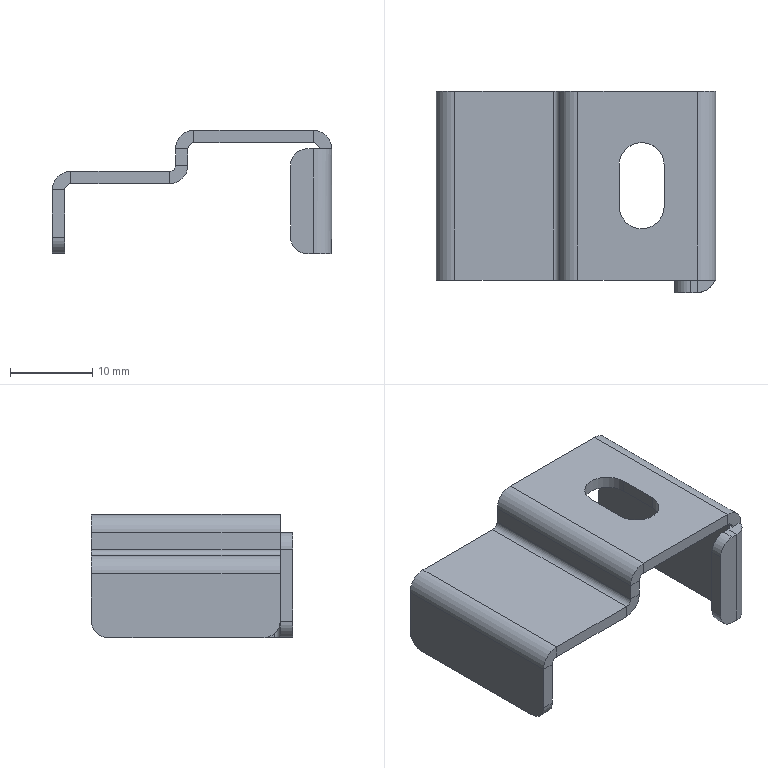Part | STEP file | 03-37 iron plate baffle A (Default) | 1 solid | 56 faces | box 34 x 24.5 x 15 mm | volume 2017 mm3 | plane 39 | cylinder 17 | commonest cylinder face diameters 1.473 x5 4 x5 4.473 x5 5.5 x2
STEP:
#1=CARTESIAN_POINT('',(9.375,-11.5,-2.237));
#2=VERTEX_POINT('',#1);
#3=CARTESIAN_POINT('',(9.5,-11.5,-2.237));
#4=VERTEX_POINT('',#3);
#5=CARTESIAN_POINT('',(8.,-11.5,-2.237));
#6=DIRECTION('',(1.,0.,0.));
#7=VECTOR('',#6,1000.);
#8=LINE('',#5,#7);
#9=EDGE_CURVE('',#2,#4,#8,.T.);
#10=ORIENTED_EDGE('',*,*,#9,.F.);
#11=CARTESIAN_POINT('',(9.5,-10.763,-2.237));
#12=VERTEX_POINT('',#11);
#13=CARTESIAN_POINT('',(7.263,-10.763,-2.237));
#14=DIRECTION('',(0.,0.,1.));
#15=DIRECTION('',(1.,0.,0.));
#16=AXIS2_PLACEMENT_3D('',#13,#14,#15);
#17=CIRCLE('',#16,2.237);
#18=EDGE_CURVE('',#2,#12,#17,.T.);
#19=ORIENTED_EDGE('',*,*,#18,.T.);
#20=CARTESIAN_POINT('',(9.5,-11.5,-2.237));
#21=DIRECTION('',(0.,1.,0.));
#22=VECTOR('',#21,1000.);
#23=LINE('',#20,#22);
#24=EDGE_CURVE('',#4,#12,#23,.T.);
#25=ORIENTED_EDGE('',*,*,#24,.F.);
#26=EDGE_LOOP('',(#10,#19,#25));
#27=FACE_OUTER_BOUND('',#26,.T.);
#28=CARTESIAN_POINT('',(8.,-11.5,-2.237));
#29=DIRECTION('',(0.,0.,-1.));
#30=DIRECTION('',(0.,1.,0.));
#31=AXIS2_PLACEMENT_3D('',#28,#29,#30);
#32=PLANE('',#31);
#33=ADVANCED_FACE('',(#27),#32,.T.);
#34=CARTESIAN_POINT('',(9.5,9.5,-15.));
#35=VERTEX_POINT('',#34);
#36=CARTESIAN_POINT('',(9.5,-10.763,-15.));
#37=VERTEX_POINT('',#36);
#38=CARTESIAN_POINT('',(9.5,-11.5,-15.));
#39=DIRECTION('',(0.,-1.,0.));
#40=VECTOR('',#39,1000.);
#41=LINE('',#38,#40);
#42=EDGE_CURVE('',#35,#37,#41,.T.);
#43=ORIENTED_EDGE('',*,*,#42,.F.);
#44=CARTESIAN_POINT('',(9.5,11.5,-13.));
#45=VERTEX_POINT('',#44);
#46=CARTESIAN_POINT('',(9.5,9.5,-13.));
#47=DIRECTION('',(1.,0.,0.));
#48=DIRECTION('',(0.,0.,-1.));
#49=AXIS2_PLACEMENT_3D('',#46,#47,#48);
#50=CIRCLE('',#49,2.);
#51=EDGE_CURVE('',#35,#45,#50,.T.);
#52=ORIENTED_EDGE('',*,*,#51,.T.);
#53=CARTESIAN_POINT('',(9.5,11.5,-2.237));
#54=VERTEX_POINT('',#53);
#55=CARTESIAN_POINT('',(9.5,11.5,-15.));
#56=DIRECTION('',(0.,0.,-1.));
#57=VECTOR('',#56,1000.);
#58=LINE('',#55,#57);
#59=EDGE_CURVE('',#54,#45,#58,.T.);
#60=ORIENTED_EDGE('',*,*,#59,.F.);
#61=CARTESIAN_POINT('',(9.5,-11.5,-2.237));
#62=DIRECTION('',(0.,-1.,0.));
#63=VECTOR('',#62,1000.);
#64=LINE('',#61,#63);
#65=EDGE_CURVE('',#54,#12,#64,.T.);
#66=ORIENTED_EDGE('',*,*,#65,.T.);
#67=CARTESIAN_POINT('',(9.5,-10.763,-2.237));
#68=DIRECTION('',(0.,0.,-1.));
#69=VECTOR('',#68,1000.);
#70=LINE('',#67,#69);
#71=EDGE_CURVE('',#12,#37,#70,.T.);
#72=ORIENTED_EDGE('',*,*,#71,.T.);
#73=EDGE_LOOP('',(#43,#52,#60,#66,#72));
#74=FACE_OUTER_BOUND('',#73,.T.);
#75=CARTESIAN_POINT('',(9.5,-11.5,-1.5));
#76=DIRECTION('',(1.,0.,0.));
#77=DIRECTION('',(0.,0.,-1.));
#78=AXIS2_PLACEMENT_3D('',#75,#76,#77);
#79=PLANE('',#78);
#80=ADVANCED_FACE('',(#74),#79,.T.);
#81=CARTESIAN_POINT('',(8.,11.5,-2.237));
#82=VERTEX_POINT('',#81);
#83=CARTESIAN_POINT('',(8.,11.5,-13.));
#84=VERTEX_POINT('',#83);
#85=CARTESIAN_POINT('',(8.,11.5,-15.));
#86=DIRECTION('',(0.,0.,-1.));
#87=VECTOR('',#86,1000.);
#88=LINE('',#85,#87);
#89=EDGE_CURVE('',#82,#84,#88,.T.);
#90=ORIENTED_EDGE('',*,*,#89,.T.);
#91=CARTESIAN_POINT('',(8.,9.5,-15.));
#92=VERTEX_POINT('',#91);
#93=CARTESIAN_POINT('',(8.,9.5,-13.));
#94=DIRECTION('',(-1.,0.,0.));
#95=DIRECTION('',(0.,0.,-1.));
#96=AXIS2_PLACEMENT_3D('',#93,#94,#95);
#97=CIRCLE('',#96,2.);
#98=EDGE_CURVE('',#84,#92,#97,.T.);
#99=ORIENTED_EDGE('',*,*,#98,.T.);
#100=CARTESIAN_POINT('',(8.,-10.763,-15.));
#101=VERTEX_POINT('',#100);
#102=CARTESIAN_POINT('',(8.,-11.5,-15.));
#103=DIRECTION('',(0.,-1.,0.));
#104=VECTOR('',#103,1000.);
#105=LINE('',#102,#104);
#106=EDGE_CURVE('',#92,#101,#105,.T.);
#107=ORIENTED_EDGE('',*,*,#106,.T.);
#108=CARTESIAN_POINT('',(8.,-10.763,-2.237));
#109=VERTEX_POINT('',#108);
#110=CARTESIAN_POINT('',(8.,-10.763,-2.237));
#111=DIRECTION('',(0.,0.,-1.));
#112=VECTOR('',#111,1000.);
#113=LINE('',#110,#112);
#114=EDGE_CURVE('',#109,#101,#113,.T.);
#115=ORIENTED_EDGE('',*,*,#114,.F.);
#116=CARTESIAN_POINT('',(8.,11.5,-2.237));
#117=DIRECTION('',(0.,-1.,0.));
#118=VECTOR('',#117,1000.);
#119=LINE('',#116,#118);
#120=EDGE_CURVE('',#82,#109,#119,.T.);
#121=ORIENTED_EDGE('',*,*,#120,.F.);
#122=EDGE_LOOP('',(#90,#99,#107,#115,#121));
#123=FACE_OUTER_BOUND('',#122,.T.);
#124=CARTESIAN_POINT('',(8.,-11.5,-1.5));
#125=DIRECTION('',(1.,0.,0.));
#126=DIRECTION('',(0.,0.,-1.));
#127=AXIS2_PLACEMENT_3D('',#124,#125,#126);
#128=PLANE('',#127);
#129=ADVANCED_FACE('',(#123),#128,.F.);
#130=CARTESIAN_POINT('',(-10.237,11.5,-6.5));
#131=VERTEX_POINT('',#130);
#132=CARTESIAN_POINT('',(-22.263,11.5,-6.5));
#133=VERTEX_POINT('',#132);
#134=CARTESIAN_POINT('',(-23.,11.5,-6.5));
#135=DIRECTION('',(-1.,0.,0.));
#136=VECTOR('',#135,1000.);
#137=LINE('',#134,#136);
#138=EDGE_CURVE('',#131,#133,#137,.T.);
#139=ORIENTED_EDGE('',*,*,#138,.T.);
#140=CARTESIAN_POINT('',(-22.263,11.5,-5.));
#141=VERTEX_POINT('',#140);
#142=CARTESIAN_POINT('',(-22.263,11.5,-6.5));
#143=DIRECTION('',(0.,0.,1.));
#144=VECTOR('',#143,1000.);
#145=LINE('',#142,#144);
#146=EDGE_CURVE('',#133,#141,#145,.T.);
#147=ORIENTED_EDGE('',*,*,#146,.T.);
#148=CARTESIAN_POINT('',(-10.237,11.5,-5.));
#149=VERTEX_POINT('',#148);
#150=CARTESIAN_POINT('',(-23.,11.5,-5.));
#151=DIRECTION('',(-1.,0.,0.));
#152=VECTOR('',#151,1000.);
#153=LINE('',#150,#152);
#154=EDGE_CURVE('',#149,#141,#153,.T.);
#155=ORIENTED_EDGE('',*,*,#154,.F.);
#156=CARTESIAN_POINT('',(-10.237,11.5,-5.));
#157=DIRECTION('',(0.,0.,-1.));
#158=VECTOR('',#157,1000.);
#159=LINE('',#156,#158);
#160=EDGE_CURVE('',#149,#131,#159,.T.);
#161=ORIENTED_EDGE('',*,*,#160,.T.);
#162=EDGE_LOOP('',(#139,#147,#155,#161));
#163=FACE_OUTER_BOUND('',#162,.T.);
#164=CARTESIAN_POINT('',(-23.,11.5,-6.5));
#165=DIRECTION('',(0.,1.,0.));
#166=DIRECTION('',(-1.,0.,0.));
#167=AXIS2_PLACEMENT_3D('',#164,#165,#166);
#168=PLANE('',#167);
#169=ADVANCED_FACE('',(#163),#168,.T.);
#170=CARTESIAN_POINT('',(-22.263,-11.5,-6.5));
#171=VERTEX_POINT('',#170);
#172=CARTESIAN_POINT('',(-10.237,-11.5,-6.5));
#173=VERTEX_POINT('',#172);
#174=CARTESIAN_POINT('',(-9.5,-11.5,-6.5));
#175=DIRECTION('',(1.,0.,0.));
#176=VECTOR('',#175,1000.);
#177=LINE('',#174,#176);
#178=EDGE_CURVE('',#171,#173,#177,.T.);
#179=ORIENTED_EDGE('',*,*,#178,.F.);
#180=CARTESIAN_POINT('',(-22.263,11.5,-6.5));
#181=DIRECTION('',(0.,-1.,0.));
#182=VECTOR('',#181,1000.);
#183=LINE('',#180,#182);
#184=EDGE_CURVE('',#133,#171,#183,.T.);
#185=ORIENTED_EDGE('',*,*,#184,.F.);
#186=ORIENTED_EDGE('',*,*,#138,.F.);
#187=CARTESIAN_POINT('',(-10.237,-11.5,-6.5));
#188=DIRECTION('',(0.,-1.,0.));
#189=VECTOR('',#188,1000.);
#190=LINE('',#187,#189);
#191=EDGE_CURVE('',#131,#173,#190,.T.);
#192=ORIENTED_EDGE('',*,*,#191,.T.);
#193=EDGE_LOOP('',(#179,#185,#186,#192));
#194=FACE_OUTER_BOUND('',#193,.T.);
#195=CARTESIAN_POINT('',(-9.5,-11.5,-6.5));
#196=DIRECTION('',(0.,0.,-1.));
#197=DIRECTION('',(-1.,0.,0.));
#198=AXIS2_PLACEMENT_3D('',#195,#196,#197);
#199=PLANE('',#198);
#200=ADVANCED_FACE('',(#194),#199,.T.);
#201=CARTESIAN_POINT('',(-22.263,-11.5,-5.));
#202=VERTEX_POINT('',#201);
#203=CARTESIAN_POINT('',(-22.263,11.5,-5.));
#204=DIRECTION('',(0.,-1.,0.));
#205=VECTOR('',#204,1000.);
#206=LINE('',#203,#205);
#207=EDGE_CURVE('',#141,#202,#206,.T.);
#208=ORIENTED_EDGE('',*,*,#207,.T.);
#209=CARTESIAN_POINT('',(-10.237,-11.5,-5.));
#210=VERTEX_POINT('',#209);
#211=CARTESIAN_POINT('',(-9.5,-11.5,-5.));
#212=DIRECTION('',(1.,0.,0.));
#213=VECTOR('',#212,1000.);
#214=LINE('',#211,#213);
#215=EDGE_CURVE('',#202,#210,#214,.T.);
#216=ORIENTED_EDGE('',*,*,#215,.T.);
#217=CARTESIAN_POINT('',(-10.237,11.5,-5.));
#218=DIRECTION('',(0.,-1.,0.));
#219=VECTOR('',#218,1000.);
#220=LINE('',#217,#219);
#221=EDGE_CURVE('',#149,#210,#220,.T.);
#222=ORIENTED_EDGE('',*,*,#221,.F.);
#223=ORIENTED_EDGE('',*,*,#154,.T.);
#224=EDGE_LOOP('',(#208,#216,#222,#223));
#225=FACE_OUTER_BOUND('',#224,.T.);
#226=CARTESIAN_POINT('',(-9.5,-11.5,-5.));
#227=DIRECTION('',(0.,0.,-1.));
#228=DIRECTION('',(-1.,0.,0.));
#229=AXIS2_PLACEMENT_3D('',#226,#227,#228);
#230=PLANE('',#229);
#231=ADVANCED_FACE('',(#225),#230,.F.);
#232=CARTESIAN_POINT('',(-9.5,-11.5,-2.237));
#233=VERTEX_POINT('',#232);
#234=CARTESIAN_POINT('',(-9.5,-11.5,-4.263));
#235=VERTEX_POINT('',#234);
#236=CARTESIAN_POINT('',(-9.5,-11.5,-5.));
#237=DIRECTION('',(0.,0.,-1.));
#238=VECTOR('',#237,1000.);
#239=LINE('',#236,#238);
#240=EDGE_CURVE('',#233,#235,#239,.T.);
#241=ORIENTED_EDGE('',*,*,#240,.T.);
#242=CARTESIAN_POINT('',(-8.,-11.5,-4.263));
#243=VERTEX_POINT('',#242);
#244=CARTESIAN_POINT('',(-9.5,-11.5,-4.263));
#245=DIRECTION('',(1.,0.,0.));
#246=VECTOR('',#245,1000.);
#247=LINE('',#244,#246);
#248=EDGE_CURVE('',#235,#243,#247,.T.);
#249=ORIENTED_EDGE('',*,*,#248,.T.);
#250=CARTESIAN_POINT('',(-8.,-11.5,-2.237));
#251=VERTEX_POINT('',#250);
#252=CARTESIAN_POINT('',(-8.,-11.5,-5.));
#253=DIRECTION('',(0.,0.,-1.));
#254=VECTOR('',#253,1000.);
#255=LINE('',#252,#254);
#256=EDGE_CURVE('',#251,#243,#255,.T.);
#257=ORIENTED_EDGE('',*,*,#256,.F.);
#258=CARTESIAN_POINT('',(-8.,-11.5,-2.237));
#259=DIRECTION('',(-1.,0.,0.));
#260=VECTOR('',#259,1000.);
#261=LINE('',#258,#260);
#262=EDGE_CURVE('',#251,#233,#261,.T.);
#263=ORIENTED_EDGE('',*,*,#262,.T.);
#264=EDGE_LOOP('',(#241,#249,#257,#263));
#265=FACE_OUTER_BOUND('',#264,.T.);
#266=CARTESIAN_POINT('',(-9.5,-11.5,-5.));
#267=DIRECTION('',(0.,-1.,0.));
#268=DIRECTION('',(1.,0.,0.));
#269=AXIS2_PLACEMENT_3D('',#266,#267,#268);
#270=PLANE('',#269);
#271=ADVANCED_FACE('',(#265),#270,.T.);
#272=CARTESIAN_POINT('',(-9.5,11.5,-4.263));
#273=VERTEX_POINT('',#272);
#274=CARTESIAN_POINT('',(-9.5,11.5,-2.237));
#275=VERTEX_POINT('',#274);
#276=CARTESIAN_POINT('',(-9.5,11.5,-1.5));
#277=DIRECTION('',(0.,0.,1.));
#278=VECTOR('',#277,1000.);
#279=LINE('',#276,#278);
#280=EDGE_CURVE('',#273,#275,#279,.T.);
#281=ORIENTED_EDGE('',*,*,#280,.F.);
#282=CARTESIAN_POINT('',(-9.5,-11.5,-4.263));
#283=DIRECTION('',(0.,1.,0.));
#284=VECTOR('',#283,1000.);
#285=LINE('',#282,#284);
#286=EDGE_CURVE('',#235,#273,#285,.T.);
#287=ORIENTED_EDGE('',*,*,#286,.F.);
#288=ORIENTED_EDGE('',*,*,#240,.F.);
#289=CARTESIAN_POINT('',(-9.5,11.5,-2.237));
#290=DIRECTION('',(0.,1.,0.));
#291=VECTOR('',#290,1000.);
#292=LINE('',#289,#291);
#293=EDGE_CURVE('',#233,#275,#292,.T.);
#294=ORIENTED_EDGE('',*,*,#293,.T.);
#295=EDGE_LOOP('',(#281,#287,#288,#294));
#296=FACE_OUTER_BOUND('',#295,.T.);
#297=CARTESIAN_POINT('',(-9.5,11.5,-1.5));
#298=DIRECTION('',(-1.,0.,0.));
#299=DIRECTION('',(0.,0.,1.));
#300=AXIS2_PLACEMENT_3D('',#297,#298,#299);
#301=PLANE('',#300);
#302=ADVANCED_FACE('',(#296),#301,.T.);
#303=CARTESIAN_POINT('',(-8.,11.5,-4.263));
#304=VERTEX_POINT('',#303);
#305=CARTESIAN_POINT('',(-8.,-11.5,-4.263));
#306=DIRECTION('',(0.,1.,0.));
#307=VECTOR('',#306,1000.);
#308=LINE('',#305,#307);
#309=EDGE_CURVE('',#243,#304,#308,.T.);
#310=ORIENTED_EDGE('',*,*,#309,.T.);
#311=CARTESIAN_POINT('',(-8.,11.5,-2.237));
#312=VERTEX_POINT('',#311);
#313=CARTESIAN_POINT('',(-8.,11.5,-1.5));
#314=DIRECTION('',(0.,0.,1.));
#315=VECTOR('',#314,1000.);
#316=LINE('',#313,#315);
#317=EDGE_CURVE('',#304,#312,#316,.T.);
#318=ORIENTED_EDGE('',*,*,#317,.T.);
#319=CARTESIAN_POINT('',(-8.,-11.5,-2.237));
#320=DIRECTION('',(0.,1.,0.));
#321=VECTOR('',#320,1000.);
#322=LINE('',#319,#321);
#323=EDGE_CURVE('',#251,#312,#322,.T.);
#324=ORIENTED_EDGE('',*,*,#323,.F.);
#325=ORIENTED_EDGE('',*,*,#256,.T.);
#326=EDGE_LOOP('',(#310,#318,#324,#325));
#327=FACE_OUTER_BOUND('',#326,.T.);
#328=CARTESIAN_POINT('',(-8.,11.5,-1.5));
#329=DIRECTION('',(-1.,0.,0.));
#330=DIRECTION('',(0.,0.,1.));
#331=AXIS2_PLACEMENT_3D('',#328,#329,#330);
#332=PLANE('',#331);
#333=ADVANCED_FACE('',(#327),#332,.F.);
#334=CARTESIAN_POINT('',(3.25,-2.5,-1.5));
#335=VERTEX_POINT('',#334);
#336=CARTESIAN_POINT('',(3.25,2.5,-1.5));
#337=VERTEX_POINT('',#336);
#338=CARTESIAN_POINT('',(3.25,-11.5,-1.5));
#339=DIRECTION('',(0.,1.,0.));
#340=VECTOR('',#339,1000.);
#341=LINE('',#338,#340);
#342=EDGE_CURVE('',#335,#337,#341,.T.);
#343=ORIENTED_EDGE('',*,*,#342,.T.);
#344=CARTESIAN_POINT('',(-2.25,2.5,-1.5));
#345=VERTEX_POINT('',#344);
#346=CARTESIAN_POINT('',(0.5,2.5,-1.5));
#347=DIRECTION('',(0.,0.,1.));
#348=DIRECTION('',(1.,0.,0.));
#349=AXIS2_PLACEMENT_3D('',#346,#347,#348);
#350=CIRCLE('',#349,2.75);
#351=EDGE_CURVE('',#337,#345,#350,.T.);
#352=ORIENTED_EDGE('',*,*,#351,.T.);
#353=CARTESIAN_POINT('',(-2.25,-2.5,-1.5));
#354=VERTEX_POINT('',#353);
#355=CARTESIAN_POINT('',(-2.25,-11.5,-1.5));
#356=DIRECTION('',(0.,-1.,0.));
#357=VECTOR('',#356,1000.);
#358=LINE('',#355,#357);
#359=EDGE_CURVE('',#345,#354,#358,.T.);
#360=ORIENTED_EDGE('',*,*,#359,.T.);
#361=CARTESIAN_POINT('',(0.5,-2.5,-1.5));
#362=DIRECTION('',(0.,0.,1.));
#363=DIRECTION('',(1.,0.,0.));
#364=AXIS2_PLACEMENT_3D('',#361,#362,#363);
#365=CIRCLE('',#364,2.75);
#366=EDGE_CURVE('',#354,#335,#365,.T.);
#367=ORIENTED_EDGE('',*,*,#366,.T.);
#368=EDGE_LOOP('',(#343,#352,#360,#367));
#369=FACE_BOUND('',#368,.T.);
#370=CARTESIAN_POINT('',(-7.263,11.5,-1.5));
#371=VERTEX_POINT('',#370);
#372=CARTESIAN_POINT('',(-7.263,-11.5,-1.5));
#373=VERTEX_POINT('',#372);
#374=CARTESIAN_POINT('',(-7.263,11.5,-1.5));
#375=DIRECTION('',(0.,-1.,0.));
#376=VECTOR('',#375,1000.);
#377=LINE('',#374,#376);
#378=EDGE_CURVE('',#371,#373,#377,.T.);
#379=ORIENTED_EDGE('',*,*,#378,.F.);
#380=CARTESIAN_POINT('',(7.263,11.5,-1.5));
#381=VERTEX_POINT('',#380);
#382=CARTESIAN_POINT('',(-8.,11.5,-1.5));
#383=DIRECTION('',(-1.,0.,0.));
#384=VECTOR('',#383,1000.);
#385=LINE('',#382,#384);
#386=EDGE_CURVE('',#381,#371,#385,.T.);
#387=ORIENTED_EDGE('',*,*,#386,.F.);
#388=CARTESIAN_POINT('',(7.263,-11.5,-1.5));
#389=VERTEX_POINT('',#388);
#390=CARTESIAN_POINT('',(7.263,-11.5,-1.5));
#391=DIRECTION('',(0.,1.,0.));
#392=VECTOR('',#391,1000.);
#393=LINE('',#390,#392);
#394=EDGE_CURVE('',#389,#381,#393,.T.);
#395=ORIENTED_EDGE('',*,*,#394,.F.);
#396=CARTESIAN_POINT('',(-8.,-11.5,-1.5));
#397=DIRECTION('',(1.,0.,0.));
#398=VECTOR('',#397,1000.);
#399=LINE('',#396,#398);
#400=EDGE_CURVE('',#373,#389,#399,.T.);
#401=ORIENTED_EDGE('',*,*,#400,.F.);
#402=EDGE_LOOP('',(#379,#387,#395,#401));
#403=FACE_OUTER_BOUND('',#402,.T.);
#404=CARTESIAN_POINT('',(8.,-11.5,-1.5));
#405=DIRECTION('',(0.,0.,1.));
#406=DIRECTION('',(1.,0.,0.));
#407=AXIS2_PLACEMENT_3D('',#404,#405,#406);
#408=PLANE('',#407);
#409=ADVANCED_FACE('',(#369,#403),#408,.F.);
#410=CARTESIAN_POINT('',(3.25,2.5,0.));
#411=VERTEX_POINT('',#410);
#412=CARTESIAN_POINT('',(-2.25,2.5,0.));
#413=VERTEX_POINT('',#412);
#414=CARTESIAN_POINT('',(0.5,2.5,0.));
#415=DIRECTION('',(0.,0.,1.));
#416=DIRECTION('',(1.,0.,0.));
#417=AXIS2_PLACEMENT_3D('',#414,#415,#416);
#418=CIRCLE('',#417,2.75);
#419=EDGE_CURVE('',#411,#413,#418,.T.);
#420=ORIENTED_EDGE('',*,*,#419,.F.);
#421=CARTESIAN_POINT('',(3.25,-2.5,0.));
#422=VERTEX_POINT('',#421);
#423=CARTESIAN_POINT('',(3.25,2.5,0.));
#424=DIRECTION('',(0.,1.,0.));
#425=VECTOR('',#424,1000.);
#426=LINE('',#423,#425);
#427=EDGE_CURVE('',#422,#411,#426,.T.);
#428=ORIENTED_EDGE('',*,*,#427,.F.);
#429=CARTESIAN_POINT('',(-2.25,-2.5,0.));
#430=VERTEX_POINT('',#429);
#431=CARTESIAN_POINT('',(0.5,-2.5,0.));
#432=DIRECTION('',(0.,0.,1.));
#433=DIRECTION('',(1.,0.,0.));
#434=AXIS2_PLACEMENT_3D('',#431,#432,#433);
#435=CIRCLE('',#434,2.75);
#436=EDGE_CURVE('',#430,#422,#435,.T.);
#437=ORIENTED_EDGE('',*,*,#436,.F.);
#438=CARTESIAN_POINT('',(-2.25,2.5,0.));
#439=DIRECTION('',(0.,-1.,0.));
#440=VECTOR('',#439,1000.);
#441=LINE('',#438,#440);
#442=EDGE_CURVE('',#413,#430,#441,.T.);
#443=ORIENTED_EDGE('',*,*,#442,.F.);
#444=EDGE_LOOP('',(#420,#428,#437,#443));
#445=FACE_BOUND('',#444,.T.);
#446=CARTESIAN_POINT('',(7.263,11.5,0.));
#447=VERTEX_POINT('',#446);
#448=CARTESIAN_POINT('',(-7.263,11.5,0.));
#449=VERTEX_POINT('',#448);
#450=CARTESIAN_POINT('',(-8.,11.5,0.));
#451=DIRECTION('',(-1.,0.,0.));
#452=VECTOR('',#451,1000.);
#453=LINE('',#450,#452);
#454=EDGE_CURVE('',#447,#449,#453,.T.);
#455=ORIENTED_EDGE('',*,*,#454,.T.);
#456=CARTESIAN_POINT('',(-7.263,-11.5,0.));
#457=VERTEX_POINT('',#456);
#458=CARTESIAN_POINT('',(-7.263,11.5,0.));
#459=DIRECTION('',(0.,-1.,0.));
#460=VECTOR('',#459,1000.);
#461=LINE('',#458,#460);
#462=EDGE_CURVE('',#449,#457,#461,.T.);
#463=ORIENTED_EDGE('',*,*,#462,.T.);
#464=CARTESIAN_POINT('',(7.263,-11.5,0.));
#465=VERTEX_POINT('',#464);
#466=CARTESIAN_POINT('',(-8.,-11.5,0.));
#467=DIRECTION('',(1.,0.,0.));
#468=VECTOR('',#467,1000.);
#469=LINE('',#466,#468);
#470=EDGE_CURVE('',#457,#465,#469,.T.);
#471=ORIENTED_EDGE('',*,*,#470,.T.);
#472=CARTESIAN_POINT('',(7.263,-11.5,0.));
#473=DIRECTION('',(0.,1.,0.));
#474=VECTOR('',#473,1000.);
#475=LINE('',#472,#474);
#476=EDGE_CURVE('',#465,#447,#475,.T.);
#477=ORIENTED_EDGE('',*,*,#476,.T.);
#478=EDGE_LOOP('',(#455,#463,#471,#477));
#479=FACE_OUTER_BOUND('',#478,.T.);
#480=CARTESIAN_POINT('',(8.,-11.5,0.));
#481=DIRECTION('',(0.,0.,1.));
#482=DIRECTION('',(1.,0.,0.));
#483=AXIS2_PLACEMENT_3D('',#480,#481,#482);
#484=PLANE('',#483);
#485=ADVANCED_FACE('',(#445,#479),#484,.T.);
#486=ORIENTED_EDGE('',*,*,#386,.T.);
#487=CARTESIAN_POINT('',(-7.263,11.5,-1.5));
#488=DIRECTION('',(0.,0.,1.));
#489=VECTOR('',#488,1000.);
#490=LINE('',#487,#489);
#491=EDGE_CURVE('',#371,#449,#490,.T.);
#492=ORIENTED_EDGE('',*,*,#491,.T.);
#493=ORIENTED_EDGE('',*,*,#454,.F.);
#494=CARTESIAN_POINT('',(7.263,11.5,-1.5));
#495=DIRECTION('',(0.,0.,1.));
#496=VECTOR('',#495,1000.);
#497=LINE('',#494,#496);
#498=EDGE_CURVE('',#381,#447,#497,.T.);
#499=ORIENTED_EDGE('',*,*,#498,.F.);
#500=EDGE_LOOP('',(#486,#492,#493,#499));
#501=FACE_OUTER_BOUND('',#500,.T.);
#502=CARTESIAN_POINT('',(-8.,11.5,-1.5));
#503=DIRECTION('',(0.,1.,0.));
#504=DIRECTION('',(0.,0.,1.));
#505=AXIS2_PLACEMENT_3D('',#502,#503,#504);
#506=PLANE('',#505);
#507=ADVANCED_FACE('',(#501),#506,.T.);
#508=CARTESIAN_POINT('',(-7.263,-11.5,-1.5));
#509=DIRECTION('',(0.,0.,1.));
#510=VECTOR('',#509,1000.);
#511=LINE('',#508,#510);
#512=EDGE_CURVE('',#373,#457,#511,.T.);
#513=ORIENTED_EDGE('',*,*,#512,.F.);
#514=ORIENTED_EDGE('',*,*,#400,.T.);
#515=CARTESIAN_POINT('',(7.263,-11.5,-1.5));
#516=DIRECTION('',(0.,0.,1.));
#517=VECTOR('',#516,1000.);
#518=LINE('',#515,#517);
#519=EDGE_CURVE('',#389,#465,#518,.T.);
#520=ORIENTED_EDGE('',*,*,#519,.T.);
#521=ORIENTED_EDGE('',*,*,#470,.F.);
#522=EDGE_LOOP('',(#513,#514,#520,#521));
#523=FACE_OUTER_BOUND('',#522,.T.);
#524=CARTESIAN_POINT('',(-8.,-11.5,-1.5));
#525=DIRECTION('',(0.,-1.,0.));
#526=DIRECTION('',(0.,0.,-1.));
#527=AXIS2_PLACEMENT_3D('',#524,#525,#526);
#528=PLANE('',#527);
#529=ADVANCED_FACE('',(#523),#528,.T.);
#530=CARTESIAN_POINT('',(8.,11.5,-2.237));
#531=DIRECTION('',(1.,0.,0.));
#532=VECTOR('',#531,1000.);
#533=LINE('',#530,#532);
#534=EDGE_CURVE('',#82,#54,#533,.T.);
#535=ORIENTED_EDGE('',*,*,#534,.F.);
#536=CARTESIAN_POINT('',(7.263,11.5,-2.237));
#537=DIRECTION('',(0.,1.,0.));
#538=DIRECTION('',(0.,0.,-1.));
#539=AXIS2_PLACEMENT_3D('',#536,#537,#538);
#540=CIRCLE('',#539,0.7366);
#541=EDGE_CURVE('',#381,#82,#540,.T.);
#542=ORIENTED_EDGE('',*,*,#541,.F.);
#543=ORIENTED_EDGE('',*,*,#498,.T.);
#544=CARTESIAN_POINT('',(7.263,11.5,-2.237));
#545=DIRECTION('',(0.,1.,0.));
#546=DIRECTION('',(0.,0.,-1.));
#547=AXIS2_PLACEMENT_3D('',#544,#545,#546);
#548=CIRCLE('',#547,2.237);
#549=EDGE_CURVE('',#447,#54,#548,.T.);
#550=ORIENTED_EDGE('',*,*,#549,.T.);
#551=EDGE_LOOP('',(#535,#542,#543,#550));
#552=FACE_OUTER_BOUND('',#551,.T.);
#553=CARTESIAN_POINT('',(7.263,11.5,-2.237));
#554=DIRECTION('',(0.,1.,0.));
#555=DIRECTION('',(0.,0.,1.));
#556=AXIS2_PLACEMENT_3D('',#553,#554,#555);
#557=PLANE('',#556);
#558=ADVANCED_FACE('',(#552),#557,.T.);
#559=CARTESIAN_POINT('',(8.,-11.5,-2.237));
#560=VERTEX_POINT('',#559);
#561=CARTESIAN_POINT('',(7.263,-11.5,-2.237));
#562=DIRECTION('',(0.,-1.,0.));
#563=DIRECTION('',(0.,0.,-1.));
#564=AXIS2_PLACEMENT_3D('',#561,#562,#563);
#565=CIRCLE('',#564,0.7366);
#566=EDGE_CURVE('',#560,#389,#565,.T.);
#567=ORIENTED_EDGE('',*,*,#566,.F.);
#568=CARTESIAN_POINT('',(8.,-11.5,-2.237));
#569=DIRECTION('',(1.,0.,0.));
#570=VECTOR('',#569,1000.);
#571=LINE('',#568,#570);
#572=EDGE_CURVE('',#560,#2,#571,.T.);
#573=ORIENTED_EDGE('',*,*,#572,.T.);
#574=ORIENTED_EDGE('',*,*,#9,.T.);
#575=CARTESIAN_POINT('',(7.263,-11.5,-2.237));
#576=DIRECTION('',(0.,-1.,0.));
#577=DIRECTION('',(0.,0.,-1.));
#578=AXIS2_PLACEMENT_3D('',#575,#576,#577);
#579=CIRCLE('',#578,2.237);
#580=EDGE_CURVE('',#4,#465,#579,.T.);
#581=ORIENTED_EDGE('',*,*,#580,.T.);
#582=ORIENTED_EDGE('',*,*,#519,.F.);
#583=EDGE_LOOP('',(#567,#573,#574,#581,#582));
#584=FACE_OUTER_BOUND('',#583,.T.);
#585=CARTESIAN_POINT('',(7.263,-11.5,-2.237));
#586=DIRECTION('',(0.,1.,0.));
#587=DIRECTION('',(0.,0.,1.));
#588=AXIS2_PLACEMENT_3D('',#585,#586,#587);
#589=PLANE('',#588);
#590=ADVANCED_FACE('',(#584),#589,.F.);
#591=ORIENTED_EDGE('',*,*,#476,.F.);
#592=ORIENTED_EDGE('',*,*,#580,.F.);
#593=ORIENTED_EDGE('',*,*,#24,.T.);
#594=ORIENTED_EDGE('',*,*,#65,.F.);
#595=ORIENTED_EDGE('',*,*,#549,.F.);
#596=EDGE_LOOP('',(#591,#592,#593,#594,#595));
#597=FACE_OUTER_BOUND('',#596,.T.);
#598=CARTESIAN_POINT('',(7.263,-11.5,-2.237));
#599=DIRECTION('',(0.,-1.,0.));
#600=DIRECTION('',(1.,0.,0.));
#601=AXIS2_PLACEMENT_3D('',#598,#599,#600);
#602=CYLINDRICAL_SURFACE('',#601,2.237);
#603=ADVANCED_FACE('',(#597),#602,.T.);
#604=ORIENTED_EDGE('',*,*,#394,.T.);
#605=ORIENTED_EDGE('',*,*,#541,.T.);
#606=ORIENTED_EDGE('',*,*,#120,.T.);
#607=CARTESIAN_POINT('',(8.,-11.5,-2.237));
#608=DIRECTION('',(0.,1.,0.));
#609=VECTOR('',#608,1000.);
#610=LINE('',#607,#609);
#611=EDGE_CURVE('',#560,#109,#610,.T.);
#612=ORIENTED_EDGE('',*,*,#611,.F.);
#613=ORIENTED_EDGE('',*,*,#566,.T.);
#614=EDGE_LOOP('',(#604,#605,#606,#612,#613));
#615=FACE_OUTER_BOUND('',#614,.T.);
#616=CARTESIAN_POINT('',(7.263,-11.5,-2.237));
#617=DIRECTION('',(0.,-1.,0.));
#618=DIRECTION('',(1.,0.,0.));
#619=AXIS2_PLACEMENT_3D('',#616,#617,#618);
#620=CYLINDRICAL_SURFACE('',#619,0.7366);
#621=ADVANCED_FACE('',(#615),#620,.F.);
#622=ORIENTED_EDGE('',*,*,#59,.T.);
#623=CARTESIAN_POINT('',(9.5,11.5,-13.));
#624=DIRECTION('',(-1.,0.,0.));
#625=VECTOR('',#624,1000.);
#626=LINE('',#623,#625);
#627=EDGE_CURVE('',#45,#84,#626,.T.);
#628=ORIENTED_EDGE('',*,*,#627,.T.);
#629=ORIENTED_EDGE('',*,*,#89,.F.);
#630=ORIENTED_EDGE('',*,*,#534,.T.);
#631=EDGE_LOOP('',(#622,#628,#629,#630));
#632=FACE_OUTER_BOUND('',#631,.T.);
#633=CARTESIAN_POINT('',(9.5,11.5,-15.));
#634=DIRECTION('',(0.,1.,0.));
#635=DIRECTION('',(-1.,0.,0.));
#636=AXIS2_PLACEMENT_3D('',#633,#634,#635);
#637=PLANE('',#636);
#638=ADVANCED_FACE('',(#632),#637,.T.);
#639=ORIENTED_EDGE('',*,*,#106,.F.);
#640=CARTESIAN_POINT('',(9.5,9.5,-15.));
#641=DIRECTION('',(1.,0.,0.));
#642=VECTOR('',#641,1000.);
#643=LINE('',#640,#642);
#644=EDGE_CURVE('',#92,#35,#643,.T.);
#645=ORIENTED_EDGE('',*,*,#644,.T.);
#646=ORIENTED_EDGE('',*,*,#42,.T.);
#647=CARTESIAN_POINT('',(8.,-10.763,-15.));
#648=DIRECTION('',(1.,0.,0.));
#649=VECTOR('',#648,1000.);
#650=LINE('',#647,#649);
#651=EDGE_CURVE('',#101,#37,#650,.T.);
#652=ORIENTED_EDGE('',*,*,#651,.F.);
#653=EDGE_LOOP('',(#639,#645,#646,#652));
#654=FACE_OUTER_BOUND('',#653,.T.);
#655=CARTESIAN_POINT('',(9.5,-11.5,-15.));
#656=DIRECTION('',(0.,0.,-1.));
#657=DIRECTION('',(-1.,0.,0.));
#658=AXIS2_PLACEMENT_3D('',#655,#656,#657);
#659=PLANE('',#658);
#660=ADVANCED_FACE('',(#654),#659,.T.);
#661=ORIENTED_EDGE('',*,*,#262,.F.);
#662=CARTESIAN_POINT('',(-7.263,-11.5,-2.237));
#663=DIRECTION('',(0.,-1.,0.));
#664=DIRECTION('',(0.,0.,1.));
#665=AXIS2_PLACEMENT_3D('',#662,#663,#664);
#666=CIRCLE('',#665,0.7366);
#667=EDGE_CURVE('',#373,#251,#666,.T.);
#668=ORIENTED_EDGE('',*,*,#667,.F.);
#669=ORIENTED_EDGE('',*,*,#512,.T.);
#670=CARTESIAN_POINT('',(-7.263,-11.5,-2.237));
#671=DIRECTION('',(0.,-1.,0.));
#672=DIRECTION('',(0.,0.,1.));
#673=AXIS2_PLACEMENT_3D('',#670,#671,#672);
#674=CIRCLE('',#673,2.237);
#675=EDGE_CURVE('',#457,#233,#674,.T.);
#676=ORIENTED_EDGE('',*,*,#675,.T.);
#677=EDGE_LOOP('',(#661,#668,#669,#676));
#678=FACE_OUTER_BOUND('',#677,.T.);
#679=CARTESIAN_POINT('',(-7.263,-11.5,-2.237));
#680=DIRECTION('',(0.,-1.,0.));
#681=DIRECTION('',(0.,0.,-1.));
#682=AXIS2_PLACEMENT_3D('',#679,#680,#681);
#683=PLANE('',#682);
#684=ADVANCED_FACE('',(#678),#683,.T.);
#685=CARTESIAN_POINT('',(-7.263,11.5,-2.237));
#686=DIRECTION('',(0.,1.,0.));
#687=DIRECTION('',(0.,0.,1.));
#688=AXIS2_PLACEMENT_3D('',#685,#686,#687);
#689=CIRCLE('',#688,0.7366);
#690=EDGE_CURVE('',#312,#371,#689,.T.);
#691=ORIENTED_EDGE('',*,*,#690,.F.);
#692=CARTESIAN_POINT('',(-8.,11.5,-2.237));
#693=DIRECTION('',(-1.,0.,0.));
#694=VECTOR('',#693,1000.);
#695=LINE('',#692,#694);
#696=EDGE_CURVE('',#312,#275,#695,.T.);
#697=ORIENTED_EDGE('',*,*,#696,.T.);
#698=CARTESIAN_POINT('',(-7.263,11.5,-2.237));
#699=DIRECTION('',(0.,1.,0.));
#700=DIRECTION('',(0.,0.,1.));
#701=AXIS2_PLACEMENT_3D('',#698,#699,#700);
#702=CIRCLE('',#701,2.237);
#703=EDGE_CURVE('',#275,#449,#702,.T.);
#704=ORIENTED_EDGE('',*,*,#703,.T.);
#705=ORIENTED_EDGE('',*,*,#491,.F.);
#706=EDGE_LOOP('',(#691,#697,#704,#705));
#707=FACE_OUTER_BOUND('',#706,.T.);
#708=CARTESIAN_POINT('',(-7.263,11.5,-2.237));
#709=DIRECTION('',(0.,-1.,0.));
#710=DIRECTION('',(0.,0.,-1.));
#711=AXIS2_PLACEMENT_3D('',#708,#709,#710);
#712=PLANE('',#711);
#713=ADVANCED_FACE('',(#707),#712,.F.);
#714=ORIENTED_EDGE('',*,*,#462,.F.);
#715=ORIENTED_EDGE('',*,*,#703,.F.);
#716=ORIENTED_EDGE('',*,*,#293,.F.);
#717=ORIENTED_EDGE('',*,*,#675,.F.);
#718=EDGE_LOOP('',(#714,#715,#716,#717));
#719=FACE_OUTER_BOUND('',#718,.T.);
#720=CARTESIAN_POINT('',(-7.263,11.5,-2.237));
#721=DIRECTION('',(0.,1.,0.));
#722=DIRECTION('',(-1.,0.,0.));
#723=AXIS2_PLACEMENT_3D('',#720,#721,#722);
#724=CYLINDRICAL_SURFACE('',#723,2.237);
#725=ADVANCED_FACE('',(#719),#724,.T.);
#726=ORIENTED_EDGE('',*,*,#378,.T.);
#727=ORIENTED_EDGE('',*,*,#667,.T.);
#728=ORIENTED_EDGE('',*,*,#323,.T.);
#729=ORIENTED_EDGE('',*,*,#690,.T.);
#730=EDGE_LOOP('',(#726,#727,#728,#729));
#731=FACE_OUTER_BOUND('',#730,.T.);
#732=CARTESIAN_POINT('',(-7.263,11.5,-2.237));
#733=DIRECTION('',(0.,1.,0.));
#734=DIRECTION('',(-1.,0.,0.));
#735=AXIS2_PLACEMENT_3D('',#732,#733,#734);
#736=CYLINDRICAL_SURFACE('',#735,0.7366);
#737=ADVANCED_FACE('',(#731),#736,.F.);
#738=CARTESIAN_POINT('',(-9.5,11.5,-4.263));
#739=DIRECTION('',(1.,0.,0.));
#740=VECTOR('',#739,1000.);
#741=LINE('',#738,#740);
#742=EDGE_CURVE('',#273,#304,#741,.T.);
#743=ORIENTED_EDGE('',*,*,#742,.F.);
#744=ORIENTED_EDGE('',*,*,#280,.T.);
#745=ORIENTED_EDGE('',*,*,#696,.F.);
#746=ORIENTED_EDGE('',*,*,#317,.F.);
#747=EDGE_LOOP('',(#743,#744,#745,#746));
#748=FACE_OUTER_BOUND('',#747,.T.);
#749=CARTESIAN_POINT('',(-9.5,11.5,-1.5));
#750=DIRECTION('',(0.,1.,0.));
#751=DIRECTION('',(-1.,0.,0.));
#752=AXIS2_PLACEMENT_3D('',#749,#750,#751);
#753=PLANE('',#752);
#754=ADVANCED_FACE('',(#748),#753,.T.);
#755=ORIENTED_EDGE('',*,*,#160,.F.);
#756=CARTESIAN_POINT('',(-10.237,11.5,-4.263));
#757=DIRECTION('',(0.,1.,0.));
#758=DIRECTION('',(0.,0.,-1.));
#759=AXIS2_PLACEMENT_3D('',#756,#757,#758);
#760=CIRCLE('',#759,0.7366);
#761=EDGE_CURVE('',#273,#149,#760,.T.);
#762=ORIENTED_EDGE('',*,*,#761,.F.);
#763=ORIENTED_EDGE('',*,*,#742,.T.);
#764=CARTESIAN_POINT('',(-10.237,11.5,-4.263));
#765=DIRECTION('',(0.,1.,0.));
#766=DIRECTION('',(0.,0.,-1.));
#767=AXIS2_PLACEMENT_3D('',#764,#765,#766);
#768=CIRCLE('',#767,2.237);
#769=EDGE_CURVE('',#304,#131,#768,.T.);
#770=ORIENTED_EDGE('',*,*,#769,.T.);
#771=EDGE_LOOP('',(#755,#762,#763,#770));
#772=FACE_OUTER_BOUND('',#771,.T.);
#773=CARTESIAN_POINT('',(-10.237,11.5,-4.263));
#774=DIRECTION('',(0.,1.,0.));
#775=DIRECTION('',(0.,0.,1.));
#776=AXIS2_PLACEMENT_3D('',#773,#774,#775);
#777=PLANE('',#776);
#778=ADVANCED_FACE('',(#772),#777,.T.);
#779=CARTESIAN_POINT('',(-10.237,-11.5,-4.263));
#780=DIRECTION('',(0.,-1.,0.));
#781=DIRECTION('',(0.,0.,-1.));
#782=AXIS2_PLACEMENT_3D('',#779,#780,#781);
#783=CIRCLE('',#782,0.7366);
#784=EDGE_CURVE('',#210,#235,#783,.T.);
#785=ORIENTED_EDGE('',*,*,#784,.F.);
#786=CARTESIAN_POINT('',(-10.237,-11.5,-5.));
#787=DIRECTION('',(0.,0.,-1.));
#788=VECTOR('',#787,1000.);
#789=LINE('',#786,#788);
#790=EDGE_CURVE('',#210,#173,#789,.T.);
#791=ORIENTED_EDGE('',*,*,#790,.T.);
#792=CARTESIAN_POINT('',(-10.237,-11.5,-4.263));
#793=DIRECTION('',(0.,-1.,0.));
#794=DIRECTION('',(0.,0.,-1.));
#795=AXIS2_PLACEMENT_3D('',#792,#793,#794);
#796=CIRCLE('',#795,2.237);
#797=EDGE_CURVE('',#173,#243,#796,.T.);
#798=ORIENTED_EDGE('',*,*,#797,.T.);
#799=ORIENTED_EDGE('',*,*,#248,.F.);
#800=EDGE_LOOP('',(#785,#791,#798,#799));
#801=FACE_OUTER_BOUND('',#800,.T.);
#802=CARTESIAN_POINT('',(-10.237,-11.5,-4.263));
#803=DIRECTION('',(0.,1.,0.));
#804=DIRECTION('',(0.,0.,1.));
#805=AXIS2_PLACEMENT_3D('',#802,#803,#804);
#806=PLANE('',#805);
#807=ADVANCED_FACE('',(#801),#806,.F.);
#808=ORIENTED_EDGE('',*,*,#309,.F.);
#809=ORIENTED_EDGE('',*,*,#797,.F.);
#810=ORIENTED_EDGE('',*,*,#191,.F.);
#811=ORIENTED_EDGE('',*,*,#769,.F.);
#812=EDGE_LOOP('',(#808,#809,#810,#811));
#813=FACE_OUTER_BOUND('',#812,.T.);
#814=CARTESIAN_POINT('',(-10.237,-11.5,-4.263));
#815=DIRECTION('',(0.,-1.,0.));
#816=DIRECTION('',(0.,0.,-1.));
#817=AXIS2_PLACEMENT_3D('',#814,#815,#816);
#818=CYLINDRICAL_SURFACE('',#817,2.237);
#819=ADVANCED_FACE('',(#813),#818,.T.);
#820=ORIENTED_EDGE('',*,*,#286,.T.);
#821=ORIENTED_EDGE('',*,*,#761,.T.);
#822=ORIENTED_EDGE('',*,*,#221,.T.);
#823=ORIENTED_EDGE('',*,*,#784,.T.);
#824=EDGE_LOOP('',(#820,#821,#822,#823));
#825=FACE_OUTER_BOUND('',#824,.T.);
#826=CARTESIAN_POINT('',(-10.237,-11.5,-4.263));
#827=DIRECTION('',(0.,-1.,0.));
#828=DIRECTION('',(0.,0.,-1.));
#829=AXIS2_PLACEMENT_3D('',#826,#827,#828);
#830=CYLINDRICAL_SURFACE('',#829,0.7366);
#831=ADVANCED_FACE('',(#825),#830,.F.);
#832=CARTESIAN_POINT('',(-22.263,-11.5,-6.5));
#833=DIRECTION('',(0.,0.,1.));
#834=VECTOR('',#833,1000.);
#835=LINE('',#832,#834);
#836=EDGE_CURVE('',#171,#202,#835,.T.);
#837=ORIENTED_EDGE('',*,*,#836,.F.);
#838=ORIENTED_EDGE('',*,*,#178,.T.);
#839=ORIENTED_EDGE('',*,*,#790,.F.);
#840=ORIENTED_EDGE('',*,*,#215,.F.);
#841=EDGE_LOOP('',(#837,#838,#839,#840));
#842=FACE_OUTER_BOUND('',#841,.T.);
#843=CARTESIAN_POINT('',(-9.5,-11.5,-6.5));
#844=DIRECTION('',(0.,-1.,0.));
#845=DIRECTION('',(1.,0.,0.));
#846=AXIS2_PLACEMENT_3D('',#843,#844,#845);
#847=PLANE('',#846);
#848=ADVANCED_FACE('',(#842),#847,.T.);
#849=CARTESIAN_POINT('',(-23.,-11.5,-7.237));
#850=VERTEX_POINT('',#849);
#851=CARTESIAN_POINT('',(-24.5,-11.5,-7.237));
#852=VERTEX_POINT('',#851);
#853=CARTESIAN_POINT('',(-23.,-11.5,-7.237));
#854=DIRECTION('',(-1.,0.,0.));
#855=VECTOR('',#854,1000.);
#856=LINE('',#853,#855);
#857=EDGE_CURVE('',#850,#852,#856,.T.);
#858=ORIENTED_EDGE('',*,*,#857,.F.);
#859=CARTESIAN_POINT('',(-22.263,-11.5,-7.237));
#860=DIRECTION('',(0.,-1.,0.));
#861=DIRECTION('',(0.,0.,1.));
#862=AXIS2_PLACEMENT_3D('',#859,#860,#861);
#863=CIRCLE('',#862,0.7366);
#864=EDGE_CURVE('',#171,#850,#863,.T.);
#865=ORIENTED_EDGE('',*,*,#864,.F.);
#866=ORIENTED_EDGE('',*,*,#836,.T.);
#867=CARTESIAN_POINT('',(-22.263,-11.5,-7.237));
#868=DIRECTION('',(0.,-1.,0.));
#869=DIRECTION('',(0.,0.,1.));
#870=AXIS2_PLACEMENT_3D('',#867,#868,#869);
#871=CIRCLE('',#870,2.237);
#872=EDGE_CURVE('',#202,#852,#871,.T.);
#873=ORIENTED_EDGE('',*,*,#872,.T.);
#874=EDGE_LOOP('',(#858,#865,#866,#873));
#875=FACE_OUTER_BOUND('',#874,.T.);
#876=CARTESIAN_POINT('',(-22.263,-11.5,-7.237));
#877=DIRECTION('',(0.,-1.,0.));
#878=DIRECTION('',(0.,0.,-1.));
#879=AXIS2_PLACEMENT_3D('',#876,#877,#878);
#880=PLANE('',#879);
#881=ADVANCED_FACE('',(#875),#880,.T.);
#882=CARTESIAN_POINT('',(-23.,11.5,-7.237));
#883=VERTEX_POINT('',#882);
#884=CARTESIAN_POINT('',(-22.263,11.5,-7.237));
#885=DIRECTION('',(0.,1.,0.));
#886=DIRECTION('',(0.,0.,1.));
#887=AXIS2_PLACEMENT_3D('',#884,#885,#886);
#888=CIRCLE('',#887,0.7366);
#889=EDGE_CURVE('',#883,#133,#888,.T.);
#890=ORIENTED_EDGE('',*,*,#889,.F.);
#891=CARTESIAN_POINT('',(-24.5,11.5,-7.237));
#892=VERTEX_POINT('',#891);
#893=CARTESIAN_POINT('',(-23.,11.5,-7.237));
#894=DIRECTION('',(-1.,0.,0.));
#895=VECTOR('',#894,1000.);
#896=LINE('',#893,#895);
#897=EDGE_CURVE('',#883,#892,#896,.T.);
#898=ORIENTED_EDGE('',*,*,#897,.T.);
#899=CARTESIAN_POINT('',(-22.263,11.5,-7.237));
#900=DIRECTION('',(0.,1.,0.));
#901=DIRECTION('',(0.,0.,1.));
#902=AXIS2_PLACEMENT_3D('',#899,#900,#901);
#903=CIRCLE('',#902,2.237);
#904=EDGE_CURVE('',#892,#141,#903,.T.);
#905=ORIENTED_EDGE('',*,*,#904,.T.);
#906=ORIENTED_EDGE('',*,*,#146,.F.);
#907=EDGE_LOOP('',(#890,#898,#905,#906));
#908=FACE_OUTER_BOUND('',#907,.T.);
#909=CARTESIAN_POINT('',(-22.263,11.5,-7.237));
#910=DIRECTION('',(0.,-1.,0.));
#911=DIRECTION('',(0.,0.,-1.));
#912=AXIS2_PLACEMENT_3D('',#909,#910,#911);
#913=PLANE('',#912);
#914=ADVANCED_FACE('',(#908),#913,.F.);
#915=ORIENTED_EDGE('',*,*,#207,.F.);
#916=ORIENTED_EDGE('',*,*,#904,.F.);
#917=CARTESIAN_POINT('',(-24.5,11.5,-7.237));
#918=DIRECTION('',(0.,1.,0.));
#919=VECTOR('',#918,1000.);
#920=LINE('',#917,#919);
#921=EDGE_CURVE('',#852,#892,#920,.T.);
#922=ORIENTED_EDGE('',*,*,#921,.F.);
#923=ORIENTED_EDGE('',*,*,#872,.F.);
#924=EDGE_LOOP('',(#915,#916,#922,#923));
#925=FACE_OUTER_BOUND('',#924,.T.);
#926=CARTESIAN_POINT('',(-22.263,11.5,-7.237));
#927=DIRECTION('',(0.,1.,0.));
#928=DIRECTION('',(-1.,0.,0.));
#929=AXIS2_PLACEMENT_3D('',#926,#927,#928);
#930=CYLINDRICAL_SURFACE('',#929,2.237);
#931=ADVANCED_FACE('',(#925),#930,.T.);
#932=ORIENTED_EDGE('',*,*,#184,.T.);
#933=ORIENTED_EDGE('',*,*,#864,.T.);
#934=CARTESIAN_POINT('',(-23.,-11.5,-7.237));
#935=DIRECTION('',(0.,1.,0.));
#936=VECTOR('',#935,1000.);
#937=LINE('',#934,#936);
#938=EDGE_CURVE('',#850,#883,#937,.T.);
#939=ORIENTED_EDGE('',*,*,#938,.T.);
#940=ORIENTED_EDGE('',*,*,#889,.T.);
#941=EDGE_LOOP('',(#932,#933,#939,#940));
#942=FACE_OUTER_BOUND('',#941,.T.);
#943=CARTESIAN_POINT('',(-22.263,11.5,-7.237));
#944=DIRECTION('',(0.,1.,0.));
#945=DIRECTION('',(-1.,0.,0.));
#946=AXIS2_PLACEMENT_3D('',#943,#944,#945);
#947=CYLINDRICAL_SURFACE('',#946,0.7366);
#948=ADVANCED_FACE('',(#942),#947,.F.);
#949=CARTESIAN_POINT('',(-23.,11.5,-13.));
#950=VERTEX_POINT('',#949);
#951=CARTESIAN_POINT('',(-23.,11.5,-6.5));
#952=DIRECTION('',(0.,0.,1.));
#953=VECTOR('',#952,1000.);
#954=LINE('',#951,#953);
#955=EDGE_CURVE('',#950,#883,#954,.T.);
#956=ORIENTED_EDGE('',*,*,#955,.F.);
#957=CARTESIAN_POINT('',(-24.5,11.5,-13.));
#958=VERTEX_POINT('',#957);
#959=CARTESIAN_POINT('',(-24.5,11.5,-13.));
#960=DIRECTION('',(-1.,0.,0.));
#961=VECTOR('',#960,1000.);
#962=LINE('',#959,#961);
#963=EDGE_CURVE('',#950,#958,#962,.T.);
#964=ORIENTED_EDGE('',*,*,#963,.T.);
#965=CARTESIAN_POINT('',(-24.5,11.5,-6.5));
#966=DIRECTION('',(0.,0.,1.));
#967=VECTOR('',#966,1000.);
#968=LINE('',#965,#967);
#969=EDGE_CURVE('',#958,#892,#968,.T.);
#970=ORIENTED_EDGE('',*,*,#969,.T.);
#971=ORIENTED_EDGE('',*,*,#897,.F.);
#972=EDGE_LOOP('',(#956,#964,#970,#971));
#973=FACE_OUTER_BOUND('',#972,.T.);
#974=CARTESIAN_POINT('',(-24.5,11.5,-6.5));
#975=DIRECTION('',(0.,1.,0.));
#976=DIRECTION('',(-1.,0.,0.));
#977=AXIS2_PLACEMENT_3D('',#974,#975,#976);
#978=PLANE('',#977);
#979=ADVANCED_FACE('',(#973),#978,.T.);
#980=CARTESIAN_POINT('',(-24.5,-11.5,-13.));
#981=VERTEX_POINT('',#980);
#982=CARTESIAN_POINT('',(-24.5,-11.5,-15.));
#983=DIRECTION('',(0.,0.,-1.));
#984=VECTOR('',#983,1000.);
#985=LINE('',#982,#984);
#986=EDGE_CURVE('',#852,#981,#985,.T.);
#987=ORIENTED_EDGE('',*,*,#986,.T.);
#988=CARTESIAN_POINT('',(-23.,-11.5,-13.));
#989=VERTEX_POINT('',#988);
#990=CARTESIAN_POINT('',(-24.5,-11.5,-13.));
#991=DIRECTION('',(1.,0.,0.));
#992=VECTOR('',#991,1000.);
#993=LINE('',#990,#992);
#994=EDGE_CURVE('',#981,#989,#993,.T.);
#995=ORIENTED_EDGE('',*,*,#994,.T.);
#996=CARTESIAN_POINT('',(-23.,-11.5,-15.));
#997=DIRECTION('',(0.,0.,-1.));
#998=VECTOR('',#997,1000.);
#999=LINE('',#996,#998);
#1000=EDGE_CURVE('',#850,#989,#999,.T.);
#1001=ORIENTED_EDGE('',*,*,#1000,.F.);
#1002=ORIENTED_EDGE('',*,*,#857,.T.);
#1003=EDGE_LOOP('',(#987,#995,#1001,#1002));
#1004=FACE_OUTER_BOUND('',#1003,.T.);
#1005=CARTESIAN_POINT('',(-24.5,-11.5,-15.));
#1006=DIRECTION('',(0.,-1.,0.));
#1007=DIRECTION('',(0.,0.,-1.));
#1008=AXIS2_PLACEMENT_3D('',#1005,#1006,#1007);
#1009=PLANE('',#1008);
#1010=ADVANCED_FACE('',(#1004),#1009,.T.);
#1011=ORIENTED_EDGE('',*,*,#969,.F.);
#1012=CARTESIAN_POINT('',(-24.5,9.5,-15.));
#1013=VERTEX_POINT('',#1012);
#1014=CARTESIAN_POINT('',(-24.5,9.5,-13.));
#1015=DIRECTION('',(-1.,0.,0.));
#1016=DIRECTION('',(0.,0.,1.));
#1017=AXIS2_PLACEMENT_3D('',#1014,#1015,#1016);
#1018=CIRCLE('',#1017,2.);
#1019=EDGE_CURVE('',#958,#1013,#1018,.T.);
#1020=ORIENTED_EDGE('',*,*,#1019,.T.);
#1021=CARTESIAN_POINT('',(-24.5,-9.5,-15.));
#1022=VERTEX_POINT('',#1021);
#1023=CARTESIAN_POINT('',(-24.5,11.5,-15.));
#1024=DIRECTION('',(0.,1.,0.));
#1025=VECTOR('',#1024,1000.);
#1026=LINE('',#1023,#1025);
#1027=EDGE_CURVE('',#1022,#1013,#1026,.T.);
#1028=ORIENTED_EDGE('',*,*,#1027,.F.);
#1029=CARTESIAN_POINT('',(-24.5,-9.5,-13.));
#1030=DIRECTION('',(-1.,0.,0.));
#1031=DIRECTION('',(0.,0.,1.));
#1032=AXIS2_PLACEMENT_3D('',#1029,#1030,#1031);
#1033=CIRCLE('',#1032,2.);
#1034=EDGE_CURVE('',#1022,#981,#1033,.T.);
#1035=ORIENTED_EDGE('',*,*,#1034,.T.);
#1036=ORIENTED_EDGE('',*,*,#986,.F.);
#1037=ORIENTED_EDGE('',*,*,#921,.T.);
#1038=EDGE_LOOP('',(#1011,#1020,#1028,#1035,#1036,#1037));
#1039=FACE_OUTER_BOUND('',#1038,.T.);
#1040=CARTESIAN_POINT('',(-24.5,11.5,-6.5));
#1041=DIRECTION('',(-1.,0.,0.));
#1042=DIRECTION('',(0.,0.,1.));
#1043=AXIS2_PLACEMENT_3D('',#1040,#1041,#1042);
#1044=PLANE('',#1043);
#1045=ADVANCED_FACE('',(#1039),#1044,.T.);
#1046=CARTESIAN_POINT('',(-23.,-9.5,-15.));
#1047=VERTEX_POINT('',#1046);
#1048=CARTESIAN_POINT('',(-23.,9.5,-15.));
#1049=VERTEX_POINT('',#1048);
#1050=CARTESIAN_POINT('',(-23.,11.5,-15.));
#1051=DIRECTION('',(0.,1.,0.));
#1052=VECTOR('',#1051,1000.);
#1053=LINE('',#1050,#1052);
#1054=EDGE_CURVE('',#1047,#1049,#1053,.T.);
#1055=ORIENTED_EDGE('',*,*,#1054,.T.);
#1056=CARTESIAN_POINT('',(-23.,9.5,-13.));
#1057=DIRECTION('',(1.,0.,0.));
#1058=DIRECTION('',(0.,0.,1.));
#1059=AXIS2_PLACEMENT_3D('',#1056,#1057,#1058);
#1060=CIRCLE('',#1059,2.);
#1061=EDGE_CURVE('',#1049,#950,#1060,.T.);
#1062=ORIENTED_EDGE('',*,*,#1061,.T.);
#1063=ORIENTED_EDGE('',*,*,#955,.T.);
#1064=ORIENTED_EDGE('',*,*,#938,.F.);
#1065=ORIENTED_EDGE('',*,*,#1000,.T.);
#1066=CARTESIAN_POINT('',(-23.,-9.5,-13.));
#1067=DIRECTION('',(1.,0.,0.));
#1068=DIRECTION('',(0.,0.,1.));
#1069=AXIS2_PLACEMENT_3D('',#1066,#1067,#1068);
#1070=CIRCLE('',#1069,2.);
#1071=EDGE_CURVE('',#989,#1047,#1070,.T.);
#1072=ORIENTED_EDGE('',*,*,#1071,.T.);
#1073=EDGE_LOOP('',(#1055,#1062,#1063,#1064,#1065,#1072));
#1074=FACE_OUTER_BOUND('',#1073,.T.);
#1075=CARTESIAN_POINT('',(-23.,11.5,-6.5));
#1076=DIRECTION('',(-1.,0.,0.));
#1077=DIRECTION('',(0.,0.,1.));
#1078=AXIS2_PLACEMENT_3D('',#1075,#1076,#1077);
#1079=PLANE('',#1078);
#1080=ADVANCED_FACE('',(#1074),#1079,.F.);
#1081=ORIENTED_EDGE('',*,*,#1027,.T.);
#1082=CARTESIAN_POINT('',(-24.5,9.5,-15.));
#1083=DIRECTION('',(1.,0.,0.));
#1084=VECTOR('',#1083,1000.);
#1085=LINE('',#1082,#1084);
#1086=EDGE_CURVE('',#1013,#1049,#1085,.T.);
#1087=ORIENTED_EDGE('',*,*,#1086,.T.);
#1088=ORIENTED_EDGE('',*,*,#1054,.F.);
#1089=CARTESIAN_POINT('',(-24.5,-9.5,-15.));
#1090=DIRECTION('',(-1.,0.,0.));
#1091=VECTOR('',#1090,1000.);
#1092=LINE('',#1089,#1091);
#1093=EDGE_CURVE('',#1047,#1022,#1092,.T.);
#1094=ORIENTED_EDGE('',*,*,#1093,.T.);
#1095=EDGE_LOOP('',(#1081,#1087,#1088,#1094));
#1096=FACE_OUTER_BOUND('',#1095,.T.);
#1097=CARTESIAN_POINT('',(-24.5,11.5,-15.));
#1098=DIRECTION('',(0.,0.,-1.));
#1099=DIRECTION('',(-1.,0.,0.));
#1100=AXIS2_PLACEMENT_3D('',#1097,#1098,#1099);
#1101=PLANE('',#1100);
#1102=ADVANCED_FACE('',(#1096),#1101,.T.);
#1103=ORIENTED_EDGE('',*,*,#572,.F.);
#1104=ORIENTED_EDGE('',*,*,#611,.T.);
#1105=CARTESIAN_POINT('',(7.263,-11.5,-2.237));
#1106=VERTEX_POINT('',#1105);
#1107=CARTESIAN_POINT('',(7.263,-10.763,-2.237));
#1108=DIRECTION('',(0.,0.,1.));
#1109=DIRECTION('',(1.,0.,0.));
#1110=AXIS2_PLACEMENT_3D('',#1107,#1108,#1109);
#1111=CIRCLE('',#1110,0.7366);
#1112=EDGE_CURVE('',#1106,#109,#1111,.T.);
#1113=ORIENTED_EDGE('',*,*,#1112,.F.);
#1114=CARTESIAN_POINT('',(7.263,-13.,-2.237));
#1115=VERTEX_POINT('',#1114);
#1116=CARTESIAN_POINT('',(7.263,-11.5,-2.237));
#1117=DIRECTION('',(0.,-1.,0.));
#1118=VECTOR('',#1117,1000.);
#1119=LINE('',#1116,#1118);
#1120=EDGE_CURVE('',#1106,#1115,#1119,.T.);
#1121=ORIENTED_EDGE('',*,*,#1120,.T.);
#1122=CARTESIAN_POINT('',(7.263,-10.763,-2.237));
#1123=DIRECTION('',(0.,0.,1.));
#1124=DIRECTION('',(1.,0.,0.));
#1125=AXIS2_PLACEMENT_3D('',#1122,#1123,#1124);
#1126=CIRCLE('',#1125,2.237);
#1127=EDGE_CURVE('',#1115,#2,#1126,.T.);
#1128=ORIENTED_EDGE('',*,*,#1127,.T.);
#1129=EDGE_LOOP('',(#1103,#1104,#1113,#1121,#1128));
#1130=FACE_OUTER_BOUND('',#1129,.T.);
#1131=CARTESIAN_POINT('',(7.263,-10.763,-2.237));
#1132=DIRECTION('',(0.,0.,-1.));
#1133=DIRECTION('',(-1.,0.,0.));
#1134=AXIS2_PLACEMENT_3D('',#1131,#1132,#1133);
#1135=PLANE('',#1134);
#1136=ADVANCED_FACE('',(#1130),#1135,.F.);
#1137=CARTESIAN_POINT('',(7.263,-11.5,-15.));
#1138=VERTEX_POINT('',#1137);
#1139=CARTESIAN_POINT('',(7.263,-13.,-15.));
#1140=VERTEX_POINT('',#1139);
#1141=CARTESIAN_POINT('',(7.263,-11.5,-15.));
#1142=DIRECTION('',(0.,-1.,0.));
#1143=VECTOR('',#1142,1000.);
#1144=LINE('',#1141,#1143);
#1145=EDGE_CURVE('',#1138,#1140,#1144,.T.);
#1146=ORIENTED_EDGE('',*,*,#1145,.F.);
#1147=CARTESIAN_POINT('',(7.263,-10.763,-15.));
#1148=DIRECTION('',(0.,0.,-1.));
#1149=DIRECTION('',(1.,0.,0.));
#1150=AXIS2_PLACEMENT_3D('',#1147,#1148,#1149);
#1151=CIRCLE('',#1150,0.7366);
#1152=EDGE_CURVE('',#101,#1138,#1151,.T.);
#1153=ORIENTED_EDGE('',*,*,#1152,.F.);
#1154=ORIENTED_EDGE('',*,*,#651,.T.);
#1155=CARTESIAN_POINT('',(7.263,-10.763,-15.));
#1156=DIRECTION('',(0.,0.,-1.));
#1157=DIRECTION('',(1.,0.,0.));
#1158=AXIS2_PLACEMENT_3D('',#1155,#1156,#1157);
#1159=CIRCLE('',#1158,2.237);
#1160=EDGE_CURVE('',#37,#1140,#1159,.T.);
#1161=ORIENTED_EDGE('',*,*,#1160,.T.);
#1162=EDGE_LOOP('',(#1146,#1153,#1154,#1161));
#1163=FACE_OUTER_BOUND('',#1162,.T.);
#1164=CARTESIAN_POINT('',(7.263,-10.763,-15.));
#1165=DIRECTION('',(0.,0.,-1.));
#1166=DIRECTION('',(-1.,0.,0.));
#1167=AXIS2_PLACEMENT_3D('',#1164,#1165,#1166);
#1168=PLANE('',#1167);
#1169=ADVANCED_FACE('',(#1163),#1168,.T.);
#1170=ORIENTED_EDGE('',*,*,#71,.F.);
#1171=ORIENTED_EDGE('',*,*,#18,.F.);
#1172=ORIENTED_EDGE('',*,*,#1127,.F.);
#1173=CARTESIAN_POINT('',(7.263,-13.,-2.237));
#1174=DIRECTION('',(0.,0.,1.));
#1175=VECTOR('',#1174,1000.);
#1176=LINE('',#1173,#1175);
#1177=EDGE_CURVE('',#1140,#1115,#1176,.T.);
#1178=ORIENTED_EDGE('',*,*,#1177,.F.);
#1179=ORIENTED_EDGE('',*,*,#1160,.F.);
#1180=EDGE_LOOP('',(#1170,#1171,#1172,#1178,#1179));
#1181=FACE_OUTER_BOUND('',#1180,.T.);
#1182=CARTESIAN_POINT('',(7.263,-10.763,-2.237));
#1183=DIRECTION('',(0.,0.,1.));
#1184=DIRECTION('',(0.,-1.,0.));
#1185=AXIS2_PLACEMENT_3D('',#1182,#1183,#1184);
#1186=CYLINDRICAL_SURFACE('',#1185,2.237);
#1187=ADVANCED_FACE('',(#1181),#1186,.T.);
#1188=ORIENTED_EDGE('',*,*,#114,.T.);
#1189=ORIENTED_EDGE('',*,*,#1152,.T.);
#1190=CARTESIAN_POINT('',(7.263,-11.5,-15.));
#1191=DIRECTION('',(0.,0.,1.));
#1192=VECTOR('',#1191,1000.);
#1193=LINE('',#1190,#1192);
#1194=EDGE_CURVE('',#1138,#1106,#1193,.T.);
#1195=ORIENTED_EDGE('',*,*,#1194,.T.);
#1196=ORIENTED_EDGE('',*,*,#1112,.T.);
#1197=EDGE_LOOP('',(#1188,#1189,#1195,#1196));
#1198=FACE_OUTER_BOUND('',#1197,.T.);
#1199=CARTESIAN_POINT('',(7.263,-10.763,-2.237));
#1200=DIRECTION('',(0.,0.,1.));
#1201=DIRECTION('',(0.,-1.,0.));
#1202=AXIS2_PLACEMENT_3D('',#1199,#1200,#1201);
#1203=CYLINDRICAL_SURFACE('',#1202,0.7366);
#1204=ADVANCED_FACE('',(#1198),#1203,.F.);
#1205=CARTESIAN_POINT('',(6.5,-11.5,-2.237));
#1206=VERTEX_POINT('',#1205);
#1207=CARTESIAN_POINT('',(8.,-11.5,-2.237));
#1208=DIRECTION('',(1.,0.,0.));
#1209=VECTOR('',#1208,1000.);
#1210=LINE('',#1207,#1209);
#1211=EDGE_CURVE('',#1206,#1106,#1210,.T.);
#1212=ORIENTED_EDGE('',*,*,#1211,.F.);
#1213=CARTESIAN_POINT('',(6.5,-13.,-2.237));
#1214=VERTEX_POINT('',#1213);
#1215=CARTESIAN_POINT('',(6.5,-13.,-2.237));
#1216=DIRECTION('',(0.,-1.,0.));
#1217=VECTOR('',#1216,1000.);
#1218=LINE('',#1215,#1217);
#1219=EDGE_CURVE('',#1206,#1214,#1218,.T.);
#1220=ORIENTED_EDGE('',*,*,#1219,.T.);
#1221=CARTESIAN_POINT('',(8.,-13.,-2.237));
#1222=DIRECTION('',(1.,0.,0.));
#1223=VECTOR('',#1222,1000.);
#1224=LINE('',#1221,#1223);
#1225=EDGE_CURVE('',#1214,#1115,#1224,.T.);
#1226=ORIENTED_EDGE('',*,*,#1225,.T.);
#1227=ORIENTED_EDGE('',*,*,#1120,.F.);
#1228=EDGE_LOOP('',(#1212,#1220,#1226,#1227));
#1229=FACE_OUTER_BOUND('',#1228,.T.);
#1230=CARTESIAN_POINT('',(8.,-13.,-2.237));
#1231=DIRECTION('',(0.,0.,1.));
#1232=DIRECTION('',(1.,0.,0.));
#1233=AXIS2_PLACEMENT_3D('',#1230,#1231,#1232);
#1234=PLANE('',#1233);
#1235=ADVANCED_FACE('',(#1229),#1234,.T.);
#1236=CARTESIAN_POINT('',(6.5,-13.,-15.));
#1237=VERTEX_POINT('',#1236);
#1238=CARTESIAN_POINT('',(4.5,-13.,-15.));
#1239=DIRECTION('',(-1.,0.,0.));
#1240=VECTOR('',#1239,1000.);
#1241=LINE('',#1238,#1240);
#1242=EDGE_CURVE('',#1140,#1237,#1241,.T.);
#1243=ORIENTED_EDGE('',*,*,#1242,.T.);
#1244=CARTESIAN_POINT('',(6.5,-11.5,-15.));
#1245=VERTEX_POINT('',#1244);
#1246=CARTESIAN_POINT('',(6.5,-13.,-15.));
#1247=DIRECTION('',(0.,1.,0.));
#1248=VECTOR('',#1247,1000.);
#1249=LINE('',#1246,#1248);
#1250=EDGE_CURVE('',#1237,#1245,#1249,.T.);
#1251=ORIENTED_EDGE('',*,*,#1250,.T.);
#1252=CARTESIAN_POINT('',(4.5,-11.5,-15.));
#1253=DIRECTION('',(-1.,0.,0.));
#1254=VECTOR('',#1253,1000.);
#1255=LINE('',#1252,#1254);
#1256=EDGE_CURVE('',#1138,#1245,#1255,.T.);
#1257=ORIENTED_EDGE('',*,*,#1256,.F.);
#1258=ORIENTED_EDGE('',*,*,#1145,.T.);
#1259=EDGE_LOOP('',(#1243,#1251,#1257,#1258));
#1260=FACE_OUTER_BOUND('',#1259,.T.);
#1261=CARTESIAN_POINT('',(4.5,-13.,-15.));
#1262=DIRECTION('',(0.,0.,-1.));
#1263=DIRECTION('',(-1.,0.,0.));
#1264=AXIS2_PLACEMENT_3D('',#1261,#1262,#1263);
#1265=PLANE('',#1264);
#1266=ADVANCED_FACE('',(#1260),#1265,.T.);
#1267=CARTESIAN_POINT('',(4.5,-13.,-13.));
#1268=VERTEX_POINT('',#1267);
#1269=CARTESIAN_POINT('',(4.5,-13.,-4.237));
#1270=VERTEX_POINT('',#1269);
#1271=CARTESIAN_POINT('',(4.5,-13.,-2.237));
#1272=DIRECTION('',(0.,0.,1.));
#1273=VECTOR('',#1272,1000.);
#1274=LINE('',#1271,#1273);
#1275=EDGE_CURVE('',#1268,#1270,#1274,.T.);
#1276=ORIENTED_EDGE('',*,*,#1275,.F.);
#1277=CARTESIAN_POINT('',(6.5,-13.,-13.));
#1278=DIRECTION('',(0.,-1.,0.));
#1279=DIRECTION('',(1.,0.,0.));
#1280=AXIS2_PLACEMENT_3D('',#1277,#1278,#1279);
#1281=CIRCLE('',#1280,2.);
#1282=EDGE_CURVE('',#1268,#1237,#1281,.T.);
#1283=ORIENTED_EDGE('',*,*,#1282,.T.);
#1284=ORIENTED_EDGE('',*,*,#1242,.F.);
#1285=ORIENTED_EDGE('',*,*,#1177,.T.);
#1286=ORIENTED_EDGE('',*,*,#1225,.F.);
#1287=CARTESIAN_POINT('',(6.5,-13.,-4.237));
#1288=DIRECTION('',(0.,-1.,0.));
#1289=DIRECTION('',(1.,0.,0.));
#1290=AXIS2_PLACEMENT_3D('',#1287,#1288,#1289);
#1291=CIRCLE('',#1290,2.);
#1292=EDGE_CURVE('',#1214,#1270,#1291,.T.);
#1293=ORIENTED_EDGE('',*,*,#1292,.T.);
#1294=EDGE_LOOP('',(#1276,#1283,#1284,#1285,#1286,#1293));
#1295=FACE_OUTER_BOUND('',#1294,.T.);
#1296=CARTESIAN_POINT('',(8.,-13.,-2.237));
#1297=DIRECTION('',(0.,-1.,0.));
#1298=DIRECTION('',(1.,0.,0.));
#1299=AXIS2_PLACEMENT_3D('',#1296,#1297,#1298);
#1300=PLANE('',#1299);
#1301=ADVANCED_FACE('',(#1295),#1300,.T.);
#1302=ORIENTED_EDGE('',*,*,#1256,.T.);
#1303=CARTESIAN_POINT('',(4.5,-11.5,-13.));
#1304=VERTEX_POINT('',#1303);
#1305=CARTESIAN_POINT('',(6.5,-11.5,-13.));
#1306=DIRECTION('',(0.,1.,0.));
#1307=DIRECTION('',(1.,0.,0.));
#1308=AXIS2_PLACEMENT_3D('',#1305,#1306,#1307);
#1309=CIRCLE('',#1308,2.);
#1310=EDGE_CURVE('',#1245,#1304,#1309,.T.);
#1311=ORIENTED_EDGE('',*,*,#1310,.T.);
#1312=CARTESIAN_POINT('',(4.5,-11.5,-4.237));
#1313=VERTEX_POINT('',#1312);
#1314=CARTESIAN_POINT('',(4.5,-11.5,-2.237));
#1315=DIRECTION('',(0.,0.,1.));
#1316=VECTOR('',#1315,1000.);
#1317=LINE('',#1314,#1316);
#1318=EDGE_CURVE('',#1304,#1313,#1317,.T.);
#1319=ORIENTED_EDGE('',*,*,#1318,.T.);
#1320=CARTESIAN_POINT('',(6.5,-11.5,-4.237));
#1321=DIRECTION('',(0.,1.,0.));
#1322=DIRECTION('',(1.,0.,0.));
#1323=AXIS2_PLACEMENT_3D('',#1320,#1321,#1322);
#1324=CIRCLE('',#1323,2.);
#1325=EDGE_CURVE('',#1313,#1206,#1324,.T.);
#1326=ORIENTED_EDGE('',*,*,#1325,.T.);
#1327=ORIENTED_EDGE('',*,*,#1211,.T.);
#1328=ORIENTED_EDGE('',*,*,#1194,.F.);
#1329=EDGE_LOOP('',(#1302,#1311,#1319,#1326,#1327,#1328));
#1330=FACE_OUTER_BOUND('',#1329,.T.);
#1331=CARTESIAN_POINT('',(8.,-11.5,-2.237));
#1332=DIRECTION('',(0.,-1.,0.));
#1333=DIRECTION('',(1.,0.,0.));
#1334=AXIS2_PLACEMENT_3D('',#1331,#1332,#1333);
#1335=PLANE('',#1334);
#1336=ADVANCED_FACE('',(#1330),#1335,.F.);
#1337=ORIENTED_EDGE('',*,*,#1318,.F.);
#1338=CARTESIAN_POINT('',(4.5,-13.,-13.));
#1339=DIRECTION('',(0.,-1.,0.));
#1340=VECTOR('',#1339,1000.);
#1341=LINE('',#1338,#1340);
#1342=EDGE_CURVE('',#1304,#1268,#1341,.T.);
#1343=ORIENTED_EDGE('',*,*,#1342,.T.);
#1344=ORIENTED_EDGE('',*,*,#1275,.T.);
#1345=CARTESIAN_POINT('',(4.5,-13.,-4.237));
#1346=DIRECTION('',(0.,1.,0.));
#1347=VECTOR('',#1346,1000.);
#1348=LINE('',#1345,#1347);
#1349=EDGE_CURVE('',#1270,#1313,#1348,.T.);
#1350=ORIENTED_EDGE('',*,*,#1349,.T.);
#1351=EDGE_LOOP('',(#1337,#1343,#1344,#1350));
#1352=FACE_OUTER_BOUND('',#1351,.T.);
#1353=CARTESIAN_POINT('',(4.5,-13.,-2.237));
#1354=DIRECTION('',(-1.,0.,0.));
#1355=DIRECTION('',(0.,0.,1.));
#1356=AXIS2_PLACEMENT_3D('',#1353,#1354,#1355);
#1357=PLANE('',#1356);
#1358=ADVANCED_FACE('',(#1352),#1357,.T.);
#1359=ORIENTED_EDGE('',*,*,#51,.F.);
#1360=ORIENTED_EDGE('',*,*,#644,.F.);
#1361=ORIENTED_EDGE('',*,*,#98,.F.);
#1362=ORIENTED_EDGE('',*,*,#627,.F.);
#1363=EDGE_LOOP('',(#1359,#1360,#1361,#1362));
#1364=FACE_OUTER_BOUND('',#1363,.T.);
#1365=CARTESIAN_POINT('',(9.5,9.5,-13.));
#1366=DIRECTION('',(-1.,0.,0.));
#1367=DIRECTION('',(0.,0.,1.));
#1368=AXIS2_PLACEMENT_3D('',#1365,#1366,#1367);
#1369=CYLINDRICAL_SURFACE('',#1368,2.);
#1370=ADVANCED_FACE('',(#1364),#1369,.T.);
#1371=ORIENTED_EDGE('',*,*,#1019,.F.);
#1372=ORIENTED_EDGE('',*,*,#963,.F.);
#1373=ORIENTED_EDGE('',*,*,#1061,.F.);
#1374=ORIENTED_EDGE('',*,*,#1086,.F.);
#1375=EDGE_LOOP('',(#1371,#1372,#1373,#1374));
#1376=FACE_OUTER_BOUND('',#1375,.T.);
#1377=CARTESIAN_POINT('',(-24.5,9.5,-13.));
#1378=DIRECTION('',(1.,0.,0.));
#1379=DIRECTION('',(0.,0.,-1.));
#1380=AXIS2_PLACEMENT_3D('',#1377,#1378,#1379);
#1381=CYLINDRICAL_SURFACE('',#1380,2.);
#1382=ADVANCED_FACE('',(#1376),#1381,.T.);
#1383=ORIENTED_EDGE('',*,*,#1034,.F.);
#1384=ORIENTED_EDGE('',*,*,#1093,.F.);
#1385=ORIENTED_EDGE('',*,*,#1071,.F.);
#1386=ORIENTED_EDGE('',*,*,#994,.F.);
#1387=EDGE_LOOP('',(#1383,#1384,#1385,#1386));
#1388=FACE_OUTER_BOUND('',#1387,.T.);
#1389=CARTESIAN_POINT('',(-24.5,-9.5,-13.));
#1390=DIRECTION('',(1.,0.,0.));
#1391=DIRECTION('',(0.,0.,-1.));
#1392=AXIS2_PLACEMENT_3D('',#1389,#1390,#1391);
#1393=CYLINDRICAL_SURFACE('',#1392,2.);
#1394=ADVANCED_FACE('',(#1388),#1393,.T.);
#1395=ORIENTED_EDGE('',*,*,#1282,.F.);
#1396=ORIENTED_EDGE('',*,*,#1342,.F.);
#1397=ORIENTED_EDGE('',*,*,#1310,.F.);
#1398=ORIENTED_EDGE('',*,*,#1250,.F.);
#1399=EDGE_LOOP('',(#1395,#1396,#1397,#1398));
#1400=FACE_OUTER_BOUND('',#1399,.T.);
#1401=CARTESIAN_POINT('',(6.5,-13.,-13.));
#1402=DIRECTION('',(0.,1.,0.));
#1403=DIRECTION('',(-1.,0.,0.));
#1404=AXIS2_PLACEMENT_3D('',#1401,#1402,#1403);
#1405=CYLINDRICAL_SURFACE('',#1404,2.);
#1406=ADVANCED_FACE('',(#1400),#1405,.T.);
#1407=ORIENTED_EDGE('',*,*,#1292,.F.);
#1408=ORIENTED_EDGE('',*,*,#1219,.F.);
#1409=ORIENTED_EDGE('',*,*,#1325,.F.);
#1410=ORIENTED_EDGE('',*,*,#1349,.F.);
#1411=EDGE_LOOP('',(#1407,#1408,#1409,#1410));
#1412=FACE_OUTER_BOUND('',#1411,.T.);
#1413=CARTESIAN_POINT('',(6.5,-13.,-4.237));
#1414=DIRECTION('',(0.,1.,0.));
#1415=DIRECTION('',(-1.,0.,0.));
#1416=AXIS2_PLACEMENT_3D('',#1413,#1414,#1415);
#1417=CYLINDRICAL_SURFACE('',#1416,2.);
#1418=ADVANCED_FACE('',(#1412),#1417,.T.);
#1419=CARTESIAN_POINT('',(3.25,2.5,-10.));
#1420=DIRECTION('',(0.,0.,1.));
#1421=VECTOR('',#1420,1000.);
#1422=LINE('',#1419,#1421);
#1423=EDGE_CURVE('',#337,#411,#1422,.T.);
#1424=ORIENTED_EDGE('',*,*,#1423,.T.);
#1425=ORIENTED_EDGE('',*,*,#419,.T.);
#1426=CARTESIAN_POINT('',(-2.25,2.5,-10.));
#1427=DIRECTION('',(0.,0.,1.));
#1428=VECTOR('',#1427,1000.);
#1429=LINE('',#1426,#1428);
#1430=EDGE_CURVE('',#345,#413,#1429,.T.);
#1431=ORIENTED_EDGE('',*,*,#1430,.F.);
#1432=ORIENTED_EDGE('',*,*,#351,.F.);
#1433=EDGE_LOOP('',(#1424,#1425,#1431,#1432));
#1434=FACE_OUTER_BOUND('',#1433,.T.);
#1435=CARTESIAN_POINT('',(0.5,2.5,-10.));
#1436=DIRECTION('',(0.,0.,1.));
#1437=DIRECTION('',(1.,0.,0.));
#1438=AXIS2_PLACEMENT_3D('',#1435,#1436,#1437);
#1439=CYLINDRICAL_SURFACE('',#1438,2.75);
#1440=ADVANCED_FACE('',(#1434),#1439,.F.);
#1441=CARTESIAN_POINT('',(3.25,-2.5,-10.));
#1442=DIRECTION('',(0.,0.,1.));
#1443=VECTOR('',#1442,1000.);
#1444=LINE('',#1441,#1443);
#1445=EDGE_CURVE('',#335,#422,#1444,.T.);
#1446=ORIENTED_EDGE('',*,*,#1445,.T.);
#1447=ORIENTED_EDGE('',*,*,#427,.T.);
#1448=ORIENTED_EDGE('',*,*,#1423,.F.);
#1449=ORIENTED_EDGE('',*,*,#342,.F.);
#1450=EDGE_LOOP('',(#1446,#1447,#1448,#1449));
#1451=FACE_OUTER_BOUND('',#1450,.T.);
#1452=CARTESIAN_POINT('',(3.25,2.5,-10.));
#1453=DIRECTION('',(1.,0.,0.));
#1454=DIRECTION('',(0.,1.,0.));
#1455=AXIS2_PLACEMENT_3D('',#1452,#1453,#1454);
#1456=PLANE('',#1455);
#1457=ADVANCED_FACE('',(#1451),#1456,.F.);
#1458=CARTESIAN_POINT('',(-2.25,-2.5,-10.));
#1459=DIRECTION('',(0.,0.,1.));
#1460=VECTOR('',#1459,1000.);
#1461=LINE('',#1458,#1460);
#1462=EDGE_CURVE('',#354,#430,#1461,.T.);
#1463=ORIENTED_EDGE('',*,*,#1462,.T.);
#1464=ORIENTED_EDGE('',*,*,#436,.T.);
#1465=ORIENTED_EDGE('',*,*,#1445,.F.);
#1466=ORIENTED_EDGE('',*,*,#366,.F.);
#1467=EDGE_LOOP('',(#1463,#1464,#1465,#1466));
#1468=FACE_OUTER_BOUND('',#1467,.T.);
#1469=CARTESIAN_POINT('',(0.5,-2.5,-10.));
#1470=DIRECTION('',(0.,0.,1.));
#1471=DIRECTION('',(1.,0.,0.));
#1472=AXIS2_PLACEMENT_3D('',#1469,#1470,#1471);
#1473=CYLINDRICAL_SURFACE('',#1472,2.75);
#1474=ADVANCED_FACE('',(#1468),#1473,.F.);
#1475=ORIENTED_EDGE('',*,*,#1430,.T.);
#1476=ORIENTED_EDGE('',*,*,#442,.T.);
#1477=ORIENTED_EDGE('',*,*,#1462,.F.);
#1478=ORIENTED_EDGE('',*,*,#359,.F.);
#1479=EDGE_LOOP('',(#1475,#1476,#1477,#1478));
#1480=FACE_OUTER_BOUND('',#1479,.T.);
#1481=CARTESIAN_POINT('',(-2.25,2.5,-10.));
#1482=DIRECTION('',(-1.,0.,0.));
#1483=DIRECTION('',(0.,-1.,0.));
#1484=AXIS2_PLACEMENT_3D('',#1481,#1482,#1483);
#1485=PLANE('',#1484);
#1486=ADVANCED_FACE('',(#1480),#1485,.F.);
#1487=CLOSED_SHELL('',(#33,#80,#129,#169,#200,#231,#271,#302,#333,#409,#485,#507,#529,#558,#590,#603,#621,#638,#660,#684,#713,#725,#737,#754,#778,#807,#819,#831,#848,#881,#914,#931,#948,#979,#1010,#1045,#1080,#1102,#1136,#1169,#1187,#1204,#1235,#1266,#1301,#1336,#1358,#1370,#1382,#1394,#1406,#1418,#1440,#1457,#1474,#1486));
#1488=MANIFOLD_SOLID_BREP('',#1487);
#1489=CARTESIAN_POINT('',(0.,0.,0.));
#1490=DIRECTION('',(0.,0.,1.));
#1491=DIRECTION('',(1.,0.,0.));
#1492=AXIS2_PLACEMENT_3D('',#1489,#1490,#1491);
#1493=(LENGTH_UNIT()NAMED_UNIT(*)SI_UNIT(.MILLI.,.METRE.));
#1494=UNCERTAINTY_MEASURE_WITH_UNIT(LENGTH_MEASURE(0.00001),#1493,'','');
#1495=(NAMED_UNIT(*)PLANE_ANGLE_UNIT()SI_UNIT($,.RADIAN.));
#1496=(NAMED_UNIT(*)SI_UNIT($,.STERADIAN.)SOLID_ANGLE_UNIT());
#1497=(GEOMETRIC_REPRESENTATION_CONTEXT(3)GLOBAL_UNCERTAINTY_ASSIGNED_CONTEXT((#1494))GLOBAL_UNIT_ASSIGNED_CONTEXT((#1493,#1495,#1496))REPRESENTATION_CONTEXT('',''));
#1498=ADVANCED_BREP_SHAPE_REPRESENTATION('',(#1488,#1492),#1497);